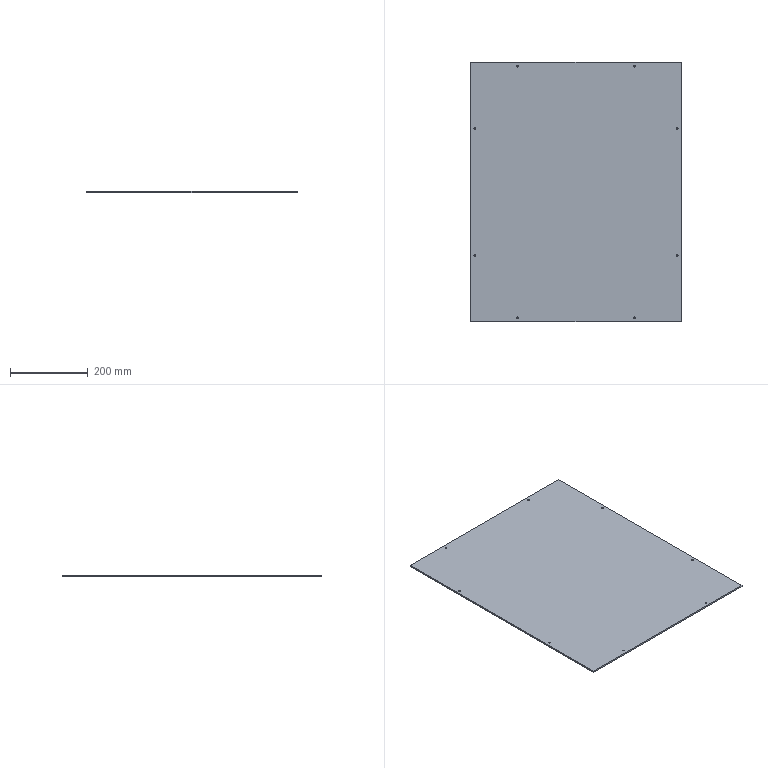Part | SolidWorks | features HoleWzd 2, MirrorPattern 2, Extrusion 1 | 1 solid | 22 faces | box 540 x 666 x 4 mm | volume 1438158 mm3 | cylinder 16 | plane 6 | commonest cylinder face diameters 4 x16
STEP:
#1=CARTESIAN_POINT('',(-258.,163.,2.));
#2=VERTEX_POINT('',#1);
#3=CARTESIAN_POINT('',(-262.,163.,2.));
#4=VERTEX_POINT('',#3);
#5=CARTESIAN_POINT('',(-260.,163.,2.));
#6=DIRECTION('',(0.,0.,-1.));
#7=DIRECTION('',(-1.,0.,0.));
#8=AXIS2_PLACEMENT_3D('',#5,#6,#7);
#9=CIRCLE('',#8,2.);
#10=EDGE_CURVE('',#2,#4,#9,.T.);
#11=ORIENTED_EDGE('',*,*,#10,.F.);
#12=CARTESIAN_POINT('',(-258.,163.,-2.));
#13=VERTEX_POINT('',#12);
#14=CARTESIAN_POINT('',(-258.,163.,-2.));
#15=DIRECTION('',(0.,0.,-1.));
#16=VECTOR('',#15,1000.);
#17=LINE('',#14,#16);
#18=EDGE_CURVE('',#2,#13,#17,.T.);
#19=ORIENTED_EDGE('',*,*,#18,.T.);
#20=CARTESIAN_POINT('',(-262.,163.,-2.));
#21=VERTEX_POINT('',#20);
#22=CARTESIAN_POINT('',(-260.,163.,-2.));
#23=DIRECTION('',(0.,0.,-1.));
#24=DIRECTION('',(-1.,0.,0.));
#25=AXIS2_PLACEMENT_3D('',#22,#23,#24);
#26=CIRCLE('',#25,2.);
#27=EDGE_CURVE('',#13,#21,#26,.T.);
#28=ORIENTED_EDGE('',*,*,#27,.T.);
#29=CARTESIAN_POINT('',(-262.,163.,-2.));
#30=DIRECTION('',(0.,0.,-1.));
#31=VECTOR('',#30,1000.);
#32=LINE('',#29,#31);
#33=EDGE_CURVE('',#4,#21,#32,.T.);
#34=ORIENTED_EDGE('',*,*,#33,.F.);
#35=EDGE_LOOP('',(#11,#19,#28,#34));
#36=FACE_OUTER_BOUND('',#35,.T.);
#37=CARTESIAN_POINT('',(-260.,163.,-2.));
#38=DIRECTION('',(0.,0.,-1.));
#39=DIRECTION('',(-1.,0.,0.));
#40=AXIS2_PLACEMENT_3D('',#37,#38,#39);
#41=CYLINDRICAL_SURFACE('',#40,2.);
#42=ADVANCED_FACE('',(#36),#41,.F.);
#43=CARTESIAN_POINT('',(-258.,-163.,2.));
#44=VERTEX_POINT('',#43);
#45=CARTESIAN_POINT('',(-262.,-163.,2.));
#46=VERTEX_POINT('',#45);
#47=CARTESIAN_POINT('',(-260.,-163.,2.));
#48=DIRECTION('',(0.,0.,-1.));
#49=DIRECTION('',(-1.,0.,0.));
#50=AXIS2_PLACEMENT_3D('',#47,#48,#49);
#51=CIRCLE('',#50,2.);
#52=EDGE_CURVE('',#44,#46,#51,.T.);
#53=ORIENTED_EDGE('',*,*,#52,.F.);
#54=CARTESIAN_POINT('',(-258.,-163.,-2.));
#55=VERTEX_POINT('',#54);
#56=CARTESIAN_POINT('',(-258.,-163.,-2.));
#57=DIRECTION('',(0.,0.,-1.));
#58=VECTOR('',#57,1000.);
#59=LINE('',#56,#58);
#60=EDGE_CURVE('',#44,#55,#59,.T.);
#61=ORIENTED_EDGE('',*,*,#60,.T.);
#62=CARTESIAN_POINT('',(-262.,-163.,-2.));
#63=VERTEX_POINT('',#62);
#64=CARTESIAN_POINT('',(-260.,-163.,-2.));
#65=DIRECTION('',(0.,0.,-1.));
#66=DIRECTION('',(-1.,0.,0.));
#67=AXIS2_PLACEMENT_3D('',#64,#65,#66);
#68=CIRCLE('',#67,2.);
#69=EDGE_CURVE('',#55,#63,#68,.T.);
#70=ORIENTED_EDGE('',*,*,#69,.T.);
#71=CARTESIAN_POINT('',(-262.,-163.,-2.));
#72=DIRECTION('',(0.,0.,-1.));
#73=VECTOR('',#72,1000.);
#74=LINE('',#71,#73);
#75=EDGE_CURVE('',#46,#63,#74,.T.);
#76=ORIENTED_EDGE('',*,*,#75,.F.);
#77=EDGE_LOOP('',(#53,#61,#70,#76));
#78=FACE_OUTER_BOUND('',#77,.T.);
#79=CARTESIAN_POINT('',(-260.,-163.,-2.));
#80=DIRECTION('',(0.,0.,-1.));
#81=DIRECTION('',(-1.,0.,0.));
#82=AXIS2_PLACEMENT_3D('',#79,#80,#81);
#83=CYLINDRICAL_SURFACE('',#82,2.);
#84=ADVANCED_FACE('',(#78),#83,.F.);
#85=CARTESIAN_POINT('',(152.,-323.,2.));
#86=VERTEX_POINT('',#85);
#87=CARTESIAN_POINT('',(148.,-323.,2.));
#88=VERTEX_POINT('',#87);
#89=CARTESIAN_POINT('',(150.,-323.,2.));
#90=DIRECTION('',(0.,0.,-1.));
#91=DIRECTION('',(-1.,0.,0.));
#92=AXIS2_PLACEMENT_3D('',#89,#90,#91);
#93=CIRCLE('',#92,2.);
#94=EDGE_CURVE('',#86,#88,#93,.T.);
#95=ORIENTED_EDGE('',*,*,#94,.F.);
#96=CARTESIAN_POINT('',(152.,-323.,-2.));
#97=VERTEX_POINT('',#96);
#98=CARTESIAN_POINT('',(152.,-323.,-2.));
#99=DIRECTION('',(0.,0.,-1.));
#100=VECTOR('',#99,1000.);
#101=LINE('',#98,#100);
#102=EDGE_CURVE('',#86,#97,#101,.T.);
#103=ORIENTED_EDGE('',*,*,#102,.T.);
#104=CARTESIAN_POINT('',(148.,-323.,-2.));
#105=VERTEX_POINT('',#104);
#106=CARTESIAN_POINT('',(150.,-323.,-2.));
#107=DIRECTION('',(0.,0.,-1.));
#108=DIRECTION('',(-1.,0.,0.));
#109=AXIS2_PLACEMENT_3D('',#106,#107,#108);
#110=CIRCLE('',#109,2.);
#111=EDGE_CURVE('',#97,#105,#110,.T.);
#112=ORIENTED_EDGE('',*,*,#111,.T.);
#113=CARTESIAN_POINT('',(148.,-323.,-2.));
#114=DIRECTION('',(0.,0.,-1.));
#115=VECTOR('',#114,1000.);
#116=LINE('',#113,#115);
#117=EDGE_CURVE('',#88,#105,#116,.T.);
#118=ORIENTED_EDGE('',*,*,#117,.F.);
#119=EDGE_LOOP('',(#95,#103,#112,#118));
#120=FACE_OUTER_BOUND('',#119,.T.);
#121=CARTESIAN_POINT('',(150.,-323.,-2.));
#122=DIRECTION('',(0.,0.,-1.));
#123=DIRECTION('',(-1.,0.,0.));
#124=AXIS2_PLACEMENT_3D('',#121,#122,#123);
#125=CYLINDRICAL_SURFACE('',#124,2.);
#126=ADVANCED_FACE('',(#120),#125,.F.);
#127=CARTESIAN_POINT('',(-148.,-323.,2.));
#128=VERTEX_POINT('',#127);
#129=CARTESIAN_POINT('',(-152.,-323.,2.));
#130=VERTEX_POINT('',#129);
#131=CARTESIAN_POINT('',(-150.,-323.,2.));
#132=DIRECTION('',(0.,0.,-1.));
#133=DIRECTION('',(-1.,0.,0.));
#134=AXIS2_PLACEMENT_3D('',#131,#132,#133);
#135=CIRCLE('',#134,2.);
#136=EDGE_CURVE('',#128,#130,#135,.T.);
#137=ORIENTED_EDGE('',*,*,#136,.F.);
#138=CARTESIAN_POINT('',(-148.,-323.,-2.));
#139=VERTEX_POINT('',#138);
#140=CARTESIAN_POINT('',(-148.,-323.,-2.));
#141=DIRECTION('',(0.,0.,-1.));
#142=VECTOR('',#141,1000.);
#143=LINE('',#140,#142);
#144=EDGE_CURVE('',#128,#139,#143,.T.);
#145=ORIENTED_EDGE('',*,*,#144,.T.);
#146=CARTESIAN_POINT('',(-152.,-323.,-2.));
#147=VERTEX_POINT('',#146);
#148=CARTESIAN_POINT('',(-150.,-323.,-2.));
#149=DIRECTION('',(0.,0.,-1.));
#150=DIRECTION('',(-1.,0.,0.));
#151=AXIS2_PLACEMENT_3D('',#148,#149,#150);
#152=CIRCLE('',#151,2.);
#153=EDGE_CURVE('',#139,#147,#152,.T.);
#154=ORIENTED_EDGE('',*,*,#153,.T.);
#155=CARTESIAN_POINT('',(-152.,-323.,-2.));
#156=DIRECTION('',(0.,0.,-1.));
#157=VECTOR('',#156,1000.);
#158=LINE('',#155,#157);
#159=EDGE_CURVE('',#130,#147,#158,.T.);
#160=ORIENTED_EDGE('',*,*,#159,.F.);
#161=EDGE_LOOP('',(#137,#145,#154,#160));
#162=FACE_OUTER_BOUND('',#161,.T.);
#163=CARTESIAN_POINT('',(-150.,-323.,-2.));
#164=DIRECTION('',(0.,0.,-1.));
#165=DIRECTION('',(-1.,0.,0.));
#166=AXIS2_PLACEMENT_3D('',#163,#164,#165);
#167=CYLINDRICAL_SURFACE('',#166,2.);
#168=ADVANCED_FACE('',(#162),#167,.F.);
#169=CARTESIAN_POINT('',(152.,323.,2.));
#170=VERTEX_POINT('',#169);
#171=CARTESIAN_POINT('',(148.,323.,2.));
#172=VERTEX_POINT('',#171);
#173=CARTESIAN_POINT('',(150.,323.,2.));
#174=DIRECTION('',(0.,0.,-1.));
#175=DIRECTION('',(-1.,0.,0.));
#176=AXIS2_PLACEMENT_3D('',#173,#174,#175);
#177=CIRCLE('',#176,2.);
#178=EDGE_CURVE('',#170,#172,#177,.T.);
#179=ORIENTED_EDGE('',*,*,#178,.F.);
#180=CARTESIAN_POINT('',(152.,323.,-2.));
#181=VERTEX_POINT('',#180);
#182=CARTESIAN_POINT('',(152.,323.,-2.));
#183=DIRECTION('',(0.,0.,-1.));
#184=VECTOR('',#183,1000.);
#185=LINE('',#182,#184);
#186=EDGE_CURVE('',#170,#181,#185,.T.);
#187=ORIENTED_EDGE('',*,*,#186,.T.);
#188=CARTESIAN_POINT('',(148.,323.,-2.));
#189=VERTEX_POINT('',#188);
#190=CARTESIAN_POINT('',(150.,323.,-2.));
#191=DIRECTION('',(0.,0.,-1.));
#192=DIRECTION('',(-1.,0.,0.));
#193=AXIS2_PLACEMENT_3D('',#190,#191,#192);
#194=CIRCLE('',#193,2.);
#195=EDGE_CURVE('',#181,#189,#194,.T.);
#196=ORIENTED_EDGE('',*,*,#195,.T.);
#197=CARTESIAN_POINT('',(148.,323.,-2.));
#198=DIRECTION('',(0.,0.,-1.));
#199=VECTOR('',#198,1000.);
#200=LINE('',#197,#199);
#201=EDGE_CURVE('',#172,#189,#200,.T.);
#202=ORIENTED_EDGE('',*,*,#201,.F.);
#203=EDGE_LOOP('',(#179,#187,#196,#202));
#204=FACE_OUTER_BOUND('',#203,.T.);
#205=CARTESIAN_POINT('',(150.,323.,-2.));
#206=DIRECTION('',(0.,0.,-1.));
#207=DIRECTION('',(-1.,0.,0.));
#208=AXIS2_PLACEMENT_3D('',#205,#206,#207);
#209=CYLINDRICAL_SURFACE('',#208,2.);
#210=ADVANCED_FACE('',(#204),#209,.F.);
#211=CARTESIAN_POINT('',(-148.,323.,2.));
#212=VERTEX_POINT('',#211);
#213=CARTESIAN_POINT('',(-152.,323.,2.));
#214=VERTEX_POINT('',#213);
#215=CARTESIAN_POINT('',(-150.,323.,2.));
#216=DIRECTION('',(0.,0.,-1.));
#217=DIRECTION('',(-1.,0.,0.));
#218=AXIS2_PLACEMENT_3D('',#215,#216,#217);
#219=CIRCLE('',#218,2.);
#220=EDGE_CURVE('',#212,#214,#219,.T.);
#221=ORIENTED_EDGE('',*,*,#220,.F.);
#222=CARTESIAN_POINT('',(-148.,323.,-2.));
#223=VERTEX_POINT('',#222);
#224=CARTESIAN_POINT('',(-148.,323.,-2.));
#225=DIRECTION('',(0.,0.,-1.));
#226=VECTOR('',#225,1000.);
#227=LINE('',#224,#226);
#228=EDGE_CURVE('',#212,#223,#227,.T.);
#229=ORIENTED_EDGE('',*,*,#228,.T.);
#230=CARTESIAN_POINT('',(-152.,323.,-2.));
#231=VERTEX_POINT('',#230);
#232=CARTESIAN_POINT('',(-150.,323.,-2.));
#233=DIRECTION('',(0.,0.,-1.));
#234=DIRECTION('',(-1.,0.,0.));
#235=AXIS2_PLACEMENT_3D('',#232,#233,#234);
#236=CIRCLE('',#235,2.);
#237=EDGE_CURVE('',#223,#231,#236,.T.);
#238=ORIENTED_EDGE('',*,*,#237,.T.);
#239=CARTESIAN_POINT('',(-152.,323.,-2.));
#240=DIRECTION('',(0.,0.,-1.));
#241=VECTOR('',#240,1000.);
#242=LINE('',#239,#241);
#243=EDGE_CURVE('',#214,#231,#242,.T.);
#244=ORIENTED_EDGE('',*,*,#243,.F.);
#245=EDGE_LOOP('',(#221,#229,#238,#244));
#246=FACE_OUTER_BOUND('',#245,.T.);
#247=CARTESIAN_POINT('',(-150.,323.,-2.));
#248=DIRECTION('',(0.,0.,-1.));
#249=DIRECTION('',(-1.,0.,0.));
#250=AXIS2_PLACEMENT_3D('',#247,#248,#249);
#251=CYLINDRICAL_SURFACE('',#250,2.);
#252=ADVANCED_FACE('',(#246),#251,.F.);
#253=CARTESIAN_POINT('',(262.,163.,2.));
#254=VERTEX_POINT('',#253);
#255=CARTESIAN_POINT('',(258.,163.,2.));
#256=VERTEX_POINT('',#255);
#257=CARTESIAN_POINT('',(260.,163.,2.));
#258=DIRECTION('',(0.,0.,-1.));
#259=DIRECTION('',(-1.,0.,0.));
#260=AXIS2_PLACEMENT_3D('',#257,#258,#259);
#261=CIRCLE('',#260,2.);
#262=EDGE_CURVE('',#254,#256,#261,.T.);
#263=ORIENTED_EDGE('',*,*,#262,.F.);
#264=CARTESIAN_POINT('',(262.,163.,-2.));
#265=VERTEX_POINT('',#264);
#266=CARTESIAN_POINT('',(262.,163.,-2.));
#267=DIRECTION('',(0.,0.,-1.));
#268=VECTOR('',#267,1000.);
#269=LINE('',#266,#268);
#270=EDGE_CURVE('',#254,#265,#269,.T.);
#271=ORIENTED_EDGE('',*,*,#270,.T.);
#272=CARTESIAN_POINT('',(258.,163.,-2.));
#273=VERTEX_POINT('',#272);
#274=CARTESIAN_POINT('',(260.,163.,-2.));
#275=DIRECTION('',(0.,0.,-1.));
#276=DIRECTION('',(-1.,0.,0.));
#277=AXIS2_PLACEMENT_3D('',#274,#275,#276);
#278=CIRCLE('',#277,2.);
#279=EDGE_CURVE('',#265,#273,#278,.T.);
#280=ORIENTED_EDGE('',*,*,#279,.T.);
#281=CARTESIAN_POINT('',(258.,163.,-2.));
#282=DIRECTION('',(0.,0.,-1.));
#283=VECTOR('',#282,1000.);
#284=LINE('',#281,#283);
#285=EDGE_CURVE('',#256,#273,#284,.T.);
#286=ORIENTED_EDGE('',*,*,#285,.F.);
#287=EDGE_LOOP('',(#263,#271,#280,#286));
#288=FACE_OUTER_BOUND('',#287,.T.);
#289=CARTESIAN_POINT('',(260.,163.,-2.));
#290=DIRECTION('',(0.,0.,-1.));
#291=DIRECTION('',(-1.,0.,0.));
#292=AXIS2_PLACEMENT_3D('',#289,#290,#291);
#293=CYLINDRICAL_SURFACE('',#292,2.);
#294=ADVANCED_FACE('',(#288),#293,.F.);
#295=CARTESIAN_POINT('',(262.,-163.,2.));
#296=VERTEX_POINT('',#295);
#297=CARTESIAN_POINT('',(258.,-163.,2.));
#298=VERTEX_POINT('',#297);
#299=CARTESIAN_POINT('',(260.,-163.,2.));
#300=DIRECTION('',(0.,0.,-1.));
#301=DIRECTION('',(-1.,0.,0.));
#302=AXIS2_PLACEMENT_3D('',#299,#300,#301);
#303=CIRCLE('',#302,2.);
#304=EDGE_CURVE('',#296,#298,#303,.T.);
#305=ORIENTED_EDGE('',*,*,#304,.F.);
#306=CARTESIAN_POINT('',(262.,-163.,-2.));
#307=VERTEX_POINT('',#306);
#308=CARTESIAN_POINT('',(262.,-163.,-2.));
#309=DIRECTION('',(0.,0.,-1.));
#310=VECTOR('',#309,1000.);
#311=LINE('',#308,#310);
#312=EDGE_CURVE('',#296,#307,#311,.T.);
#313=ORIENTED_EDGE('',*,*,#312,.T.);
#314=CARTESIAN_POINT('',(258.,-163.,-2.));
#315=VERTEX_POINT('',#314);
#316=CARTESIAN_POINT('',(260.,-163.,-2.));
#317=DIRECTION('',(0.,0.,-1.));
#318=DIRECTION('',(-1.,0.,0.));
#319=AXIS2_PLACEMENT_3D('',#316,#317,#318);
#320=CIRCLE('',#319,2.);
#321=EDGE_CURVE('',#307,#315,#320,.T.);
#322=ORIENTED_EDGE('',*,*,#321,.T.);
#323=CARTESIAN_POINT('',(258.,-163.,-2.));
#324=DIRECTION('',(0.,0.,-1.));
#325=VECTOR('',#324,1000.);
#326=LINE('',#323,#325);
#327=EDGE_CURVE('',#298,#315,#326,.T.);
#328=ORIENTED_EDGE('',*,*,#327,.F.);
#329=EDGE_LOOP('',(#305,#313,#322,#328));
#330=FACE_OUTER_BOUND('',#329,.T.);
#331=CARTESIAN_POINT('',(260.,-163.,-2.));
#332=DIRECTION('',(0.,0.,-1.));
#333=DIRECTION('',(-1.,0.,0.));
#334=AXIS2_PLACEMENT_3D('',#331,#332,#333);
#335=CYLINDRICAL_SURFACE('',#334,2.);
#336=ADVANCED_FACE('',(#330),#335,.F.);
#337=CARTESIAN_POINT('',(270.,-333.,-2.));
#338=VERTEX_POINT('',#337);
#339=CARTESIAN_POINT('',(270.,333.,-2.));
#340=VERTEX_POINT('',#339);
#341=CARTESIAN_POINT('',(270.,-333.,-2.));
#342=DIRECTION('',(0.,1.,0.));
#343=VECTOR('',#342,1000.);
#344=LINE('',#341,#343);
#345=EDGE_CURVE('',#338,#340,#344,.T.);
#346=ORIENTED_EDGE('',*,*,#345,.T.);
#347=CARTESIAN_POINT('',(270.,333.,2.));
#348=VERTEX_POINT('',#347);
#349=CARTESIAN_POINT('',(270.,333.,2.));
#350=DIRECTION('',(0.,0.,-1.));
#351=VECTOR('',#350,1000.);
#352=LINE('',#349,#351);
#353=EDGE_CURVE('',#348,#340,#352,.T.);
#354=ORIENTED_EDGE('',*,*,#353,.F.);
#355=CARTESIAN_POINT('',(270.,-333.,2.));
#356=VERTEX_POINT('',#355);
#357=CARTESIAN_POINT('',(270.,-333.,2.));
#358=DIRECTION('',(0.,1.,0.));
#359=VECTOR('',#358,1000.);
#360=LINE('',#357,#359);
#361=EDGE_CURVE('',#356,#348,#360,.T.);
#362=ORIENTED_EDGE('',*,*,#361,.F.);
#363=CARTESIAN_POINT('',(270.,-333.,2.));
#364=DIRECTION('',(0.,0.,-1.));
#365=VECTOR('',#364,1000.);
#366=LINE('',#363,#365);
#367=EDGE_CURVE('',#356,#338,#366,.T.);
#368=ORIENTED_EDGE('',*,*,#367,.T.);
#369=EDGE_LOOP('',(#346,#354,#362,#368));
#370=FACE_OUTER_BOUND('',#369,.T.);
#371=CARTESIAN_POINT('',(270.,-333.,2.));
#372=DIRECTION('',(-1.,0.,0.));
#373=DIRECTION('',(0.,0.,1.));
#374=AXIS2_PLACEMENT_3D('',#371,#372,#373);
#375=PLANE('',#374);
#376=ADVANCED_FACE('',(#370),#375,.F.);
#377=CARTESIAN_POINT('',(-270.,333.,-2.));
#378=VERTEX_POINT('',#377);
#379=CARTESIAN_POINT('',(-270.,333.,-2.));
#380=DIRECTION('',(-1.,0.,0.));
#381=VECTOR('',#380,1000.);
#382=LINE('',#379,#381);
#383=EDGE_CURVE('',#340,#378,#382,.T.);
#384=ORIENTED_EDGE('',*,*,#383,.T.);
#385=CARTESIAN_POINT('',(-270.,333.,2.));
#386=VERTEX_POINT('',#385);
#387=CARTESIAN_POINT('',(-270.,333.,2.));
#388=DIRECTION('',(0.,0.,-1.));
#389=VECTOR('',#388,1000.);
#390=LINE('',#387,#389);
#391=EDGE_CURVE('',#386,#378,#390,.T.);
#392=ORIENTED_EDGE('',*,*,#391,.F.);
#393=CARTESIAN_POINT('',(-270.,333.,2.));
#394=DIRECTION('',(-1.,0.,0.));
#395=VECTOR('',#394,1000.);
#396=LINE('',#393,#395);
#397=EDGE_CURVE('',#348,#386,#396,.T.);
#398=ORIENTED_EDGE('',*,*,#397,.F.);
#399=ORIENTED_EDGE('',*,*,#353,.T.);
#400=EDGE_LOOP('',(#384,#392,#398,#399));
#401=FACE_OUTER_BOUND('',#400,.T.);
#402=CARTESIAN_POINT('',(-270.,333.,2.));
#403=DIRECTION('',(0.,-1.,0.));
#404=DIRECTION('',(0.,0.,-1.));
#405=AXIS2_PLACEMENT_3D('',#402,#403,#404);
#406=PLANE('',#405);
#407=ADVANCED_FACE('',(#401),#406,.F.);
#408=CARTESIAN_POINT('',(-270.,-333.,-2.));
#409=VERTEX_POINT('',#408);
#410=CARTESIAN_POINT('',(-270.,-333.,-2.));
#411=DIRECTION('',(0.,-1.,0.));
#412=VECTOR('',#411,1000.);
#413=LINE('',#410,#412);
#414=EDGE_CURVE('',#378,#409,#413,.T.);
#415=ORIENTED_EDGE('',*,*,#414,.T.);
#416=CARTESIAN_POINT('',(-270.,-333.,2.));
#417=VERTEX_POINT('',#416);
#418=CARTESIAN_POINT('',(-270.,-333.,2.));
#419=DIRECTION('',(0.,0.,-1.));
#420=VECTOR('',#419,1000.);
#421=LINE('',#418,#420);
#422=EDGE_CURVE('',#417,#409,#421,.T.);
#423=ORIENTED_EDGE('',*,*,#422,.F.);
#424=CARTESIAN_POINT('',(-270.,-333.,2.));
#425=DIRECTION('',(0.,-1.,0.));
#426=VECTOR('',#425,1000.);
#427=LINE('',#424,#426);
#428=EDGE_CURVE('',#386,#417,#427,.T.);
#429=ORIENTED_EDGE('',*,*,#428,.F.);
#430=ORIENTED_EDGE('',*,*,#391,.T.);
#431=EDGE_LOOP('',(#415,#423,#429,#430));
#432=FACE_OUTER_BOUND('',#431,.T.);
#433=CARTESIAN_POINT('',(-270.,-333.,2.));
#434=DIRECTION('',(1.,0.,0.));
#435=DIRECTION('',(0.,0.,-1.));
#436=AXIS2_PLACEMENT_3D('',#433,#434,#435);
#437=PLANE('',#436);
#438=ADVANCED_FACE('',(#432),#437,.F.);
#439=CARTESIAN_POINT('',(-270.,-333.,-2.));
#440=DIRECTION('',(1.,0.,0.));
#441=VECTOR('',#440,1000.);
#442=LINE('',#439,#441);
#443=EDGE_CURVE('',#409,#338,#442,.T.);
#444=ORIENTED_EDGE('',*,*,#443,.T.);
#445=ORIENTED_EDGE('',*,*,#367,.F.);
#446=CARTESIAN_POINT('',(-270.,-333.,2.));
#447=DIRECTION('',(1.,0.,0.));
#448=VECTOR('',#447,1000.);
#449=LINE('',#446,#448);
#450=EDGE_CURVE('',#417,#356,#449,.T.);
#451=ORIENTED_EDGE('',*,*,#450,.F.);
#452=ORIENTED_EDGE('',*,*,#422,.T.);
#453=EDGE_LOOP('',(#444,#445,#451,#452));
#454=FACE_OUTER_BOUND('',#453,.T.);
#455=CARTESIAN_POINT('',(-270.,-333.,2.));
#456=DIRECTION('',(0.,1.,0.));
#457=DIRECTION('',(0.,0.,1.));
#458=AXIS2_PLACEMENT_3D('',#455,#456,#457);
#459=PLANE('',#458);
#460=ADVANCED_FACE('',(#454),#459,.F.);
#461=CARTESIAN_POINT('',(-260.,163.,2.));
#462=DIRECTION('',(0.,0.,-1.));
#463=DIRECTION('',(-1.,0.,0.));
#464=AXIS2_PLACEMENT_3D('',#461,#462,#463);
#465=CIRCLE('',#464,2.);
#466=EDGE_CURVE('',#4,#2,#465,.T.);
#467=ORIENTED_EDGE('',*,*,#466,.T.);
#468=ORIENTED_EDGE('',*,*,#10,.T.);
#469=EDGE_LOOP('',(#467,#468));
#470=FACE_BOUND('',#469,.T.);
#471=CARTESIAN_POINT('',(-260.,-163.,2.));
#472=DIRECTION('',(0.,0.,-1.));
#473=DIRECTION('',(-1.,0.,0.));
#474=AXIS2_PLACEMENT_3D('',#471,#472,#473);
#475=CIRCLE('',#474,2.);
#476=EDGE_CURVE('',#46,#44,#475,.T.);
#477=ORIENTED_EDGE('',*,*,#476,.T.);
#478=ORIENTED_EDGE('',*,*,#52,.T.);
#479=EDGE_LOOP('',(#477,#478));
#480=FACE_BOUND('',#479,.T.);
#481=CARTESIAN_POINT('',(150.,-323.,2.));
#482=DIRECTION('',(0.,0.,-1.));
#483=DIRECTION('',(-1.,0.,0.));
#484=AXIS2_PLACEMENT_3D('',#481,#482,#483);
#485=CIRCLE('',#484,2.);
#486=EDGE_CURVE('',#88,#86,#485,.T.);
#487=ORIENTED_EDGE('',*,*,#486,.T.);
#488=ORIENTED_EDGE('',*,*,#94,.T.);
#489=EDGE_LOOP('',(#487,#488));
#490=FACE_BOUND('',#489,.T.);
#491=CARTESIAN_POINT('',(-150.,-323.,2.));
#492=DIRECTION('',(0.,0.,-1.));
#493=DIRECTION('',(-1.,0.,0.));
#494=AXIS2_PLACEMENT_3D('',#491,#492,#493);
#495=CIRCLE('',#494,2.);
#496=EDGE_CURVE('',#130,#128,#495,.T.);
#497=ORIENTED_EDGE('',*,*,#496,.T.);
#498=ORIENTED_EDGE('',*,*,#136,.T.);
#499=EDGE_LOOP('',(#497,#498));
#500=FACE_BOUND('',#499,.T.);
#501=CARTESIAN_POINT('',(150.,323.,2.));
#502=DIRECTION('',(0.,0.,-1.));
#503=DIRECTION('',(-1.,0.,0.));
#504=AXIS2_PLACEMENT_3D('',#501,#502,#503);
#505=CIRCLE('',#504,2.);
#506=EDGE_CURVE('',#172,#170,#505,.T.);
#507=ORIENTED_EDGE('',*,*,#506,.T.);
#508=ORIENTED_EDGE('',*,*,#178,.T.);
#509=EDGE_LOOP('',(#507,#508));
#510=FACE_BOUND('',#509,.T.);
#511=CARTESIAN_POINT('',(-150.,323.,2.));
#512=DIRECTION('',(0.,0.,-1.));
#513=DIRECTION('',(-1.,0.,0.));
#514=AXIS2_PLACEMENT_3D('',#511,#512,#513);
#515=CIRCLE('',#514,2.);
#516=EDGE_CURVE('',#214,#212,#515,.T.);
#517=ORIENTED_EDGE('',*,*,#516,.T.);
#518=ORIENTED_EDGE('',*,*,#220,.T.);
#519=EDGE_LOOP('',(#517,#518));
#520=FACE_BOUND('',#519,.T.);
#521=CARTESIAN_POINT('',(260.,163.,2.));
#522=DIRECTION('',(0.,0.,-1.));
#523=DIRECTION('',(-1.,0.,0.));
#524=AXIS2_PLACEMENT_3D('',#521,#522,#523);
#525=CIRCLE('',#524,2.);
#526=EDGE_CURVE('',#256,#254,#525,.T.);
#527=ORIENTED_EDGE('',*,*,#526,.T.);
#528=ORIENTED_EDGE('',*,*,#262,.T.);
#529=EDGE_LOOP('',(#527,#528));
#530=FACE_BOUND('',#529,.T.);
#531=CARTESIAN_POINT('',(260.,-163.,2.));
#532=DIRECTION('',(0.,0.,-1.));
#533=DIRECTION('',(-1.,0.,0.));
#534=AXIS2_PLACEMENT_3D('',#531,#532,#533);
#535=CIRCLE('',#534,2.);
#536=EDGE_CURVE('',#298,#296,#535,.T.);
#537=ORIENTED_EDGE('',*,*,#536,.T.);
#538=ORIENTED_EDGE('',*,*,#304,.T.);
#539=EDGE_LOOP('',(#537,#538));
#540=FACE_BOUND('',#539,.T.);
#541=ORIENTED_EDGE('',*,*,#361,.T.);
#542=ORIENTED_EDGE('',*,*,#397,.T.);
#543=ORIENTED_EDGE('',*,*,#428,.T.);
#544=ORIENTED_EDGE('',*,*,#450,.T.);
#545=EDGE_LOOP('',(#541,#542,#543,#544));
#546=FACE_OUTER_BOUND('',#545,.T.);
#547=CARTESIAN_POINT('',(0.,0.,2.));
#548=DIRECTION('',(0.,0.,-1.));
#549=DIRECTION('',(-1.,0.,0.));
#550=AXIS2_PLACEMENT_3D('',#547,#548,#549);
#551=PLANE('',#550);
#552=ADVANCED_FACE('',(#470,#480,#490,#500,#510,#520,#530,#540,#546),#551,.F.);
#553=CARTESIAN_POINT('',(-260.,163.,-2.));
#554=DIRECTION('',(0.,0.,-1.));
#555=DIRECTION('',(-1.,0.,0.));
#556=AXIS2_PLACEMENT_3D('',#553,#554,#555);
#557=CIRCLE('',#556,2.);
#558=EDGE_CURVE('',#21,#13,#557,.T.);
#559=ORIENTED_EDGE('',*,*,#558,.F.);
#560=ORIENTED_EDGE('',*,*,#27,.F.);
#561=EDGE_LOOP('',(#559,#560));
#562=FACE_BOUND('',#561,.T.);
#563=CARTESIAN_POINT('',(-260.,-163.,-2.));
#564=DIRECTION('',(0.,0.,-1.));
#565=DIRECTION('',(-1.,0.,0.));
#566=AXIS2_PLACEMENT_3D('',#563,#564,#565);
#567=CIRCLE('',#566,2.);
#568=EDGE_CURVE('',#63,#55,#567,.T.);
#569=ORIENTED_EDGE('',*,*,#568,.F.);
#570=ORIENTED_EDGE('',*,*,#69,.F.);
#571=EDGE_LOOP('',(#569,#570));
#572=FACE_BOUND('',#571,.T.);
#573=CARTESIAN_POINT('',(150.,-323.,-2.));
#574=DIRECTION('',(0.,0.,-1.));
#575=DIRECTION('',(-1.,0.,0.));
#576=AXIS2_PLACEMENT_3D('',#573,#574,#575);
#577=CIRCLE('',#576,2.);
#578=EDGE_CURVE('',#105,#97,#577,.T.);
#579=ORIENTED_EDGE('',*,*,#578,.F.);
#580=ORIENTED_EDGE('',*,*,#111,.F.);
#581=EDGE_LOOP('',(#579,#580));
#582=FACE_BOUND('',#581,.T.);
#583=CARTESIAN_POINT('',(-150.,-323.,-2.));
#584=DIRECTION('',(0.,0.,-1.));
#585=DIRECTION('',(-1.,0.,0.));
#586=AXIS2_PLACEMENT_3D('',#583,#584,#585);
#587=CIRCLE('',#586,2.);
#588=EDGE_CURVE('',#147,#139,#587,.T.);
#589=ORIENTED_EDGE('',*,*,#588,.F.);
#590=ORIENTED_EDGE('',*,*,#153,.F.);
#591=EDGE_LOOP('',(#589,#590));
#592=FACE_BOUND('',#591,.T.);
#593=CARTESIAN_POINT('',(150.,323.,-2.));
#594=DIRECTION('',(0.,0.,-1.));
#595=DIRECTION('',(-1.,0.,0.));
#596=AXIS2_PLACEMENT_3D('',#593,#594,#595);
#597=CIRCLE('',#596,2.);
#598=EDGE_CURVE('',#189,#181,#597,.T.);
#599=ORIENTED_EDGE('',*,*,#598,.F.);
#600=ORIENTED_EDGE('',*,*,#195,.F.);
#601=EDGE_LOOP('',(#599,#600));
#602=FACE_BOUND('',#601,.T.);
#603=CARTESIAN_POINT('',(-150.,323.,-2.));
#604=DIRECTION('',(0.,0.,-1.));
#605=DIRECTION('',(-1.,0.,0.));
#606=AXIS2_PLACEMENT_3D('',#603,#604,#605);
#607=CIRCLE('',#606,2.);
#608=EDGE_CURVE('',#231,#223,#607,.T.);
#609=ORIENTED_EDGE('',*,*,#608,.F.);
#610=ORIENTED_EDGE('',*,*,#237,.F.);
#611=EDGE_LOOP('',(#609,#610));
#612=FACE_BOUND('',#611,.T.);
#613=CARTESIAN_POINT('',(260.,163.,-2.));
#614=DIRECTION('',(0.,0.,-1.));
#615=DIRECTION('',(-1.,0.,0.));
#616=AXIS2_PLACEMENT_3D('',#613,#614,#615);
#617=CIRCLE('',#616,2.);
#618=EDGE_CURVE('',#273,#265,#617,.T.);
#619=ORIENTED_EDGE('',*,*,#618,.F.);
#620=ORIENTED_EDGE('',*,*,#279,.F.);
#621=EDGE_LOOP('',(#619,#620));
#622=FACE_BOUND('',#621,.T.);
#623=CARTESIAN_POINT('',(260.,-163.,-2.));
#624=DIRECTION('',(0.,0.,-1.));
#625=DIRECTION('',(-1.,0.,0.));
#626=AXIS2_PLACEMENT_3D('',#623,#624,#625);
#627=CIRCLE('',#626,2.);
#628=EDGE_CURVE('',#315,#307,#627,.T.);
#629=ORIENTED_EDGE('',*,*,#628,.F.);
#630=ORIENTED_EDGE('',*,*,#321,.F.);
#631=EDGE_LOOP('',(#629,#630));
#632=FACE_BOUND('',#631,.T.);
#633=ORIENTED_EDGE('',*,*,#345,.F.);
#634=ORIENTED_EDGE('',*,*,#443,.F.);
#635=ORIENTED_EDGE('',*,*,#414,.F.);
#636=ORIENTED_EDGE('',*,*,#383,.F.);
#637=EDGE_LOOP('',(#633,#634,#635,#636));
#638=FACE_OUTER_BOUND('',#637,.T.);
#639=CARTESIAN_POINT('',(0.,0.,-2.));
#640=DIRECTION('',(0.,0.,-1.));
#641=DIRECTION('',(-1.,0.,0.));
#642=AXIS2_PLACEMENT_3D('',#639,#640,#641);
#643=PLANE('',#642);
#644=ADVANCED_FACE('',(#562,#572,#582,#592,#602,#612,#622,#632,#638),#643,.T.);
#645=ORIENTED_EDGE('',*,*,#312,.F.);
#646=ORIENTED_EDGE('',*,*,#536,.F.);
#647=ORIENTED_EDGE('',*,*,#327,.T.);
#648=ORIENTED_EDGE('',*,*,#628,.T.);
#649=EDGE_LOOP('',(#645,#646,#647,#648));
#650=FACE_OUTER_BOUND('',#649,.T.);
#651=CARTESIAN_POINT('',(260.,-163.,-2.));
#652=DIRECTION('',(0.,0.,-1.));
#653=DIRECTION('',(-1.,0.,0.));
#654=AXIS2_PLACEMENT_3D('',#651,#652,#653);
#655=CYLINDRICAL_SURFACE('',#654,2.);
#656=ADVANCED_FACE('',(#650),#655,.F.);
#657=ORIENTED_EDGE('',*,*,#270,.F.);
#658=ORIENTED_EDGE('',*,*,#526,.F.);
#659=ORIENTED_EDGE('',*,*,#285,.T.);
#660=ORIENTED_EDGE('',*,*,#618,.T.);
#661=EDGE_LOOP('',(#657,#658,#659,#660));
#662=FACE_OUTER_BOUND('',#661,.T.);
#663=CARTESIAN_POINT('',(260.,163.,-2.));
#664=DIRECTION('',(0.,0.,-1.));
#665=DIRECTION('',(-1.,0.,0.));
#666=AXIS2_PLACEMENT_3D('',#663,#664,#665);
#667=CYLINDRICAL_SURFACE('',#666,2.);
#668=ADVANCED_FACE('',(#662),#667,.F.);
#669=ORIENTED_EDGE('',*,*,#228,.F.);
#670=ORIENTED_EDGE('',*,*,#516,.F.);
#671=ORIENTED_EDGE('',*,*,#243,.T.);
#672=ORIENTED_EDGE('',*,*,#608,.T.);
#673=EDGE_LOOP('',(#669,#670,#671,#672));
#674=FACE_OUTER_BOUND('',#673,.T.);
#675=CARTESIAN_POINT('',(-150.,323.,-2.));
#676=DIRECTION('',(0.,0.,-1.));
#677=DIRECTION('',(-1.,0.,0.));
#678=AXIS2_PLACEMENT_3D('',#675,#676,#677);
#679=CYLINDRICAL_SURFACE('',#678,2.);
#680=ADVANCED_FACE('',(#674),#679,.F.);
#681=ORIENTED_EDGE('',*,*,#186,.F.);
#682=ORIENTED_EDGE('',*,*,#506,.F.);
#683=ORIENTED_EDGE('',*,*,#201,.T.);
#684=ORIENTED_EDGE('',*,*,#598,.T.);
#685=EDGE_LOOP('',(#681,#682,#683,#684));
#686=FACE_OUTER_BOUND('',#685,.T.);
#687=CARTESIAN_POINT('',(150.,323.,-2.));
#688=DIRECTION('',(0.,0.,-1.));
#689=DIRECTION('',(-1.,0.,0.));
#690=AXIS2_PLACEMENT_3D('',#687,#688,#689);
#691=CYLINDRICAL_SURFACE('',#690,2.);
#692=ADVANCED_FACE('',(#686),#691,.F.);
#693=ORIENTED_EDGE('',*,*,#144,.F.);
#694=ORIENTED_EDGE('',*,*,#496,.F.);
#695=ORIENTED_EDGE('',*,*,#159,.T.);
#696=ORIENTED_EDGE('',*,*,#588,.T.);
#697=EDGE_LOOP('',(#693,#694,#695,#696));
#698=FACE_OUTER_BOUND('',#697,.T.);
#699=CARTESIAN_POINT('',(-150.,-323.,-2.));
#700=DIRECTION('',(0.,0.,-1.));
#701=DIRECTION('',(-1.,0.,0.));
#702=AXIS2_PLACEMENT_3D('',#699,#700,#701);
#703=CYLINDRICAL_SURFACE('',#702,2.);
#704=ADVANCED_FACE('',(#698),#703,.F.);
#705=ORIENTED_EDGE('',*,*,#102,.F.);
#706=ORIENTED_EDGE('',*,*,#486,.F.);
#707=ORIENTED_EDGE('',*,*,#117,.T.);
#708=ORIENTED_EDGE('',*,*,#578,.T.);
#709=EDGE_LOOP('',(#705,#706,#707,#708));
#710=FACE_OUTER_BOUND('',#709,.T.);
#711=CARTESIAN_POINT('',(150.,-323.,-2.));
#712=DIRECTION('',(0.,0.,-1.));
#713=DIRECTION('',(-1.,0.,0.));
#714=AXIS2_PLACEMENT_3D('',#711,#712,#713);
#715=CYLINDRICAL_SURFACE('',#714,2.);
#716=ADVANCED_FACE('',(#710),#715,.F.);
#717=ORIENTED_EDGE('',*,*,#60,.F.);
#718=ORIENTED_EDGE('',*,*,#476,.F.);
#719=ORIENTED_EDGE('',*,*,#75,.T.);
#720=ORIENTED_EDGE('',*,*,#568,.T.);
#721=EDGE_LOOP('',(#717,#718,#719,#720));
#722=FACE_OUTER_BOUND('',#721,.T.);
#723=CARTESIAN_POINT('',(-260.,-163.,-2.));
#724=DIRECTION('',(0.,0.,-1.));
#725=DIRECTION('',(-1.,0.,0.));
#726=AXIS2_PLACEMENT_3D('',#723,#724,#725);
#727=CYLINDRICAL_SURFACE('',#726,2.);
#728=ADVANCED_FACE('',(#722),#727,.F.);
#729=ORIENTED_EDGE('',*,*,#18,.F.);
#730=ORIENTED_EDGE('',*,*,#466,.F.);
#731=ORIENTED_EDGE('',*,*,#33,.T.);
#732=ORIENTED_EDGE('',*,*,#558,.T.);
#733=EDGE_LOOP('',(#729,#730,#731,#732));
#734=FACE_OUTER_BOUND('',#733,.T.);
#735=CARTESIAN_POINT('',(-260.,163.,-2.));
#736=DIRECTION('',(0.,0.,-1.));
#737=DIRECTION('',(-1.,0.,0.));
#738=AXIS2_PLACEMENT_3D('',#735,#736,#737);
#739=CYLINDRICAL_SURFACE('',#738,2.);
#740=ADVANCED_FACE('',(#734),#739,.F.);
#741=CLOSED_SHELL('',(#42,#84,#126,#168,#210,#252,#294,#336,#376,#407,#438,#460,#552,#644,#656,#668,#680,#692,#704,#716,#728,#740));
#742=MANIFOLD_SOLID_BREP('',#741);
#743=CARTESIAN_POINT('',(0.,0.,0.));
#744=DIRECTION('',(0.,0.,1.));
#745=DIRECTION('',(1.,0.,0.));
#746=AXIS2_PLACEMENT_3D('',#743,#744,#745);
#747=(LENGTH_UNIT()NAMED_UNIT(*)SI_UNIT(.MILLI.,.METRE.));
#748=UNCERTAINTY_MEASURE_WITH_UNIT(LENGTH_MEASURE(0.00001),#747,'','');
#749=(NAMED_UNIT(*)PLANE_ANGLE_UNIT()SI_UNIT($,.RADIAN.));
#750=(NAMED_UNIT(*)SI_UNIT($,.STERADIAN.)SOLID_ANGLE_UNIT());
#751=(GEOMETRIC_REPRESENTATION_CONTEXT(3)GLOBAL_UNCERTAINTY_ASSIGNED_CONTEXT((#748))GLOBAL_UNIT_ASSIGNED_CONTEXT((#747,#749,#750))REPRESENTATION_CONTEXT('',''));
#752=ADVANCED_BREP_SHAPE_REPRESENTATION('',(#742,#746),#751);